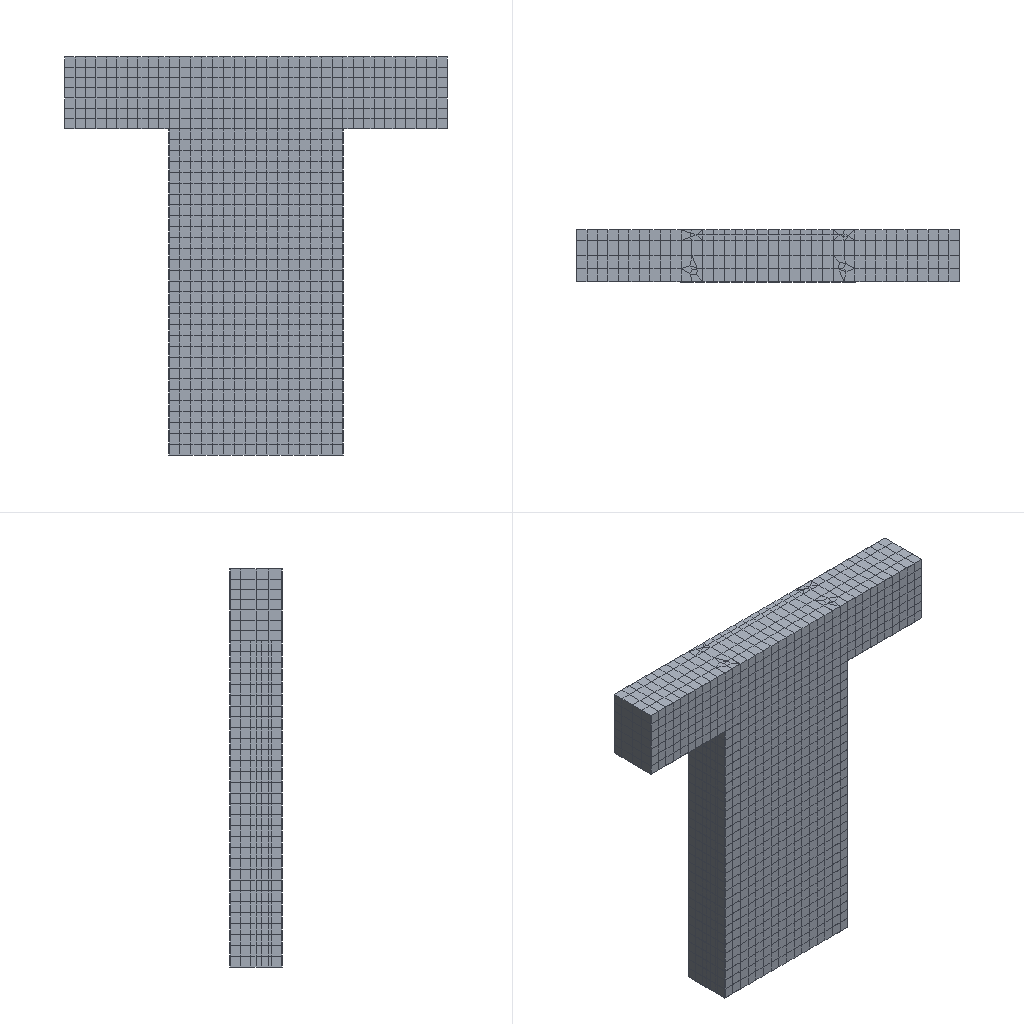Simulation study | abaqus
Set-up summary:
category,name,step,type,value,unit,region
solver,abaqus
solver,version,,,Abaqus/Standard 2020
units,not stated in the deck,,not stated
analysis,deck,,static,static
load_step,Step-1,Step-1,static
load_step,Step-2,Step-2,static
load_step,requested,,,2
mesh,nodes,,,11062
mesh,elements,,,8420
element_type,C3D6,,solid,444
element_type,R3D4,,rigid,1002
element_type,T3D2,,truss,2018
element_type,C3D8R,,solid,4956
load,load commands in deck,,count,2
bc,support commands in deck,,count,7
material,CON,,in results
material,Q235,,in results
check,setup vs results,,match,"per instance, exact: element labels, types and connectivity; labels of the nodes the elements use; coordinates of those nodes at SINGLE_PRECISION in 3 of 6 instance(s)"
Abaqus input file, long lists of numbers shortened:
*Heading
** Job name: Job-2 Model name: Model-1-Copy
** Generated by: Abaqus/CAE 2020
*Preprint, echo=NO, model=NO, history=NO, contact=NO
**
** PARTS
**
*Part, name=ban1
*Node
      1,         189.,         220.,           0.
      2,         189.,        -180.,           0.
** (494 more lines like these left out)
*Element, type=R3D4
1,  1, 13, 24,  4
2, 13, 14, 23, 24
** (499 more lines like these left out)
*Node
    497,         189.,          20.,          -5.
*Nset, nset=ban1-RefPt_, internal
497,
*Elset, elset=ban1, generate
   1,  501,    1
*End Part
**
*Part, name=ban2
*Node
      1,         189.,         220.,        1835.
      2,         189.,        -180.,        1835.
** (494 more lines like these left out)
*Element, type=R3D4
1,  1, 13, 24,  4
2, 13, 14, 23, 24
** (499 more lines like these left out)
*Node
    497,         189.,          20.,        1830.
*Nset, nset=ban2-RefPt_, internal
497,
*Elset, elset=ban2, generate
   1,  501,    1
*End Part
**
*Part, name=con
*Node
      1,         489.,          90.,        1500.
      2,        -111.,          90.,        1500.
** (5932 more lines like these left out)
*Element, type=C3D8R
  1,    5, 1585,  129,    1, 1654, 3925, 3903, 1653
  2, 1585, 1586,  130,  129, 3925, 3926, 3904, 3903
** (3814 more lines like these left out)
*Element, type=C3D6
1093,    5,   23,    1,  345,  546,  307
1094, 2438,   27,   28, 4466,  439,  547
** (442 more lines like these left out)
*Nset, nset=Set-12
    1,    2,    3,    4,    5,    6,    7,    8,    9,   10,   11,   12,   13,   14,   15,   16
   17,   18,   19,   20,   21,   22,   23,   24,   25,   26,   27,   28,   29,   30,   31,   32
** (360 more lines like these left out)
*Elset, elset=Set-12
    1,    2,    3,    4,    5,    6,    7,    8,    9,   10,   11,   12,   13,   14,   15,   16
   17,   18,   19,   20,   21,   22,   23,   24,   25,   26,   27,   28,   29,   30,   31,   32
** (249 more lines like these left out)
*Nset, nset=Set-14, generate
    1,  5934,     1
*Elset, elset=Set-14, generate
    1,  4260,     1
** Section: con
*Solid Section, elset=Set-14, material=con
,
*End Part
**
*Part, name=fiber
*Node
      1,         734.,          52.,        1525.
      2,         734.,         115.,        1525.
** (1652 more lines like these left out)
*Element, type=T3D2
1, 2, 1
2,   3, 873
** (2016 more lines like these left out)
*Nset, nset=Set-3, generate
    1,  1654,     1
*Elset, elset=Set-3, generate
    1,  2018,     1
*Nset, nset=nei
    1,    2,    3,    4,    5,    6,    7,    8,    9,   10,   11,   12,   13,   14,   15,   16
   17,   18,   19,   20,   21,   22,   23,   24,   25,   26,   27,   28,   29,   30,   31,   32
** (39 more lines like these left out)
*Elset, elset=nei
    1,    2,    3,    4,    5,    6,    7,    8,    9,   10,   11,   12,   13,   14,   15,   16
   17,   18,   19,   20,   21,   22,   23,   24,   25,   26,   27,   28,   29,   30,   31,   32
** (45 more lines like these left out)
** Section: fiber
*Solid Section, elset=Set-3, material=q235
12.56,
*End Part
**
*Part, name=liang1
*Node
      1,         588.,         140.,        1500.
      2,         588.,         140.,           0.
** (1238 more lines like these left out)
*Element, type=C3D8R
 1,   8, 145, 922, 176,   1,  57, 893, 116
 2, 145, 144, 923, 922,  57,  58, 894, 893
** (568 more lines like these left out)
*Nset, nset=Set-1, generate
    1,  1240,     1
*Elset, elset=Set-1, generate
   1,  570,    1
** Section: liang
*Solid Section, elset=Set-1, material=q235
,
*End Part
**
*Part, name=liang2
*Node
      1,        -112.,         -99.,           0.
      2,        -112.,         -99.,        1500.
** (1238 more lines like these left out)
*Element, type=C3D8R
 1, 174, 893, 922, 173,   1,  57, 114,   4
 2, 893, 894, 923, 922,  57,  58, 113, 114
** (568 more lines like these left out)
*Nset, nset=Set-1, generate
    1,  1240,     1
*Elset, elset=Set-1, generate
   1,  570,    1
** Section: liang
*Solid Section, elset=Set-1, material=q235
,
*End Part
**
**
** ASSEMBLY
**
*Assembly, name=Assembly
**
*Instance, name=ban1-1, part=ban1
*End Instance
**
*Instance, name=ban2-1, part=ban2
*End Instance
**
*Instance, name=con-1, part=con
*End Instance
**
*Instance, name=fiber-1, part=fiber
*End Instance
**
*Instance, name=liang1-1, part=liang1
*End Instance
**
*Instance, name=liang2-1, part=liang2
*End Instance
**
*Nset, nset=Set-4, instance=ban2-1
 497,
*Nset, nset=Set-5, instance=ban1-1
 497,
*Nset, nset=Set-6, instance=ban1-1
 497,
*Nset, nset=insert, instance=fiber-1
    1,    2,    3,    4,    5,    6,    7,    8,    9,   10,   11,   12,   13,   14,   15,   16
   17,   18,   19,   20,   21,   22,   23,   24,   25,   26,   27,   28,   29,   30,   31,   32
** (42 more lines like these left out)
*Nset, nset=m_Set-6, instance=fiber-1
    1,    2,    3,    4,    5,    6,    7,    8,    9,   10,   11,   12,   13,   14,   15,   16
   17,   18,   19,   20,   21,   22,   23,   24,   25,   26,   27,   28,   29,   30,   31,   32
** (40 more lines like these left out)
*Elset, elset=m_Set-6, instance=fiber-1
    1,    2,    3,    4,    5,    6,    7,    8,    9,   10,   11,   12,   13,   14,   15,   16
   17,   18,   19,   20,   21,   22,   23,   24,   25,   26,   27,   28,   29,   30,   31,   32
** (48 more lines like these left out)
*Nset, nset=m_Set-8, instance=fiber-1
    1,    2,    3,    4,    5,    6,    7,    8,    9,   10,   11,   12,   13,   14,   15,   16
   17,   18,   19,   20,   21,   22,   23,   24,   25,   26,   27,   28,   29,   30,   31,   32
** (38 more lines like these left out)
*Elset, elset=m_Set-8, instance=fiber-1
    1,    2,    3,    4,    5,    6,    7,    8,    9,   10,   11,   12,   13,   14,   15,   16
   17,   18,   19,   20,   21,   22,   23,   24,   25,   26,   27,   28,   29,   30,   31,   32
** (45 more lines like these left out)
*Nset, nset=m_Set-10, instance=fiber-1
    1,    2,    3,    4,    5,    6,    7,    8,    9,   10,   11,   12,   13,   14,   15,   16
   17,   18,   19,   20,   21,   22,   23,   24,   25,   26,   27,   28,   29,   30,   31,   32
** (38 more lines like these left out)
*Elset, elset=m_Set-10, instance=fiber-1
    1,    2,    3,    4,    5,    6,    7,    8,    9,   10,   11,   12,   13,   14,   15,   16
   17,   18,   19,   20,   21,   22,   23,   24,   25,   26,   27,   28,   29,   30,   31,   32
** (45 more lines like these left out)
*Nset, nset=m_Set-12, instance=fiber-1
    1,    2,    3,    4,    5,    6,    7,    8,    9,   10,   11,   12,   13,   14,   15,   16
   17,   18,   19,   20,   21,   22,   23,   24,   25,   26,   27,   28,   29,   30,   31,   32
** (91 more lines like these left out)
*Elset, elset=m_Set-12, instance=fiber-1
    1,    2,    3,    4,    5,    6,    7,    8,    9,   10,   11,   12,   13,   14,   15,   16
   17,   18,   19,   20,   21,   22,   23,   24,   25,   26,   27,   28,   29,   30,   31,   32
** (110 more lines like these left out)
*Nset, nset=s_Set-6, instance=con-1
    1,    2,    3,    4,    5,    6,    7,    8,    9,   10,   11,   12,   13,   14,   15,   16
   17,   18,   19,   20,   21,   22,   23,   24,   25,   26,   27,   28,   29,   30,   31,   32
** (360 more lines like these left out)
*Elset, elset=s_Set-6, instance=con-1
    1,    2,    3,    4,    5,    6,    7,    8,    9,   10,   11,   12,   13,   14,   15,   16
   17,   18,   19,   20,   21,   22,   23,   24,   25,   26,   27,   28,   29,   30,   31,   32
** (249 more lines like these left out)
*Nset, nset=s_Set-10, instance=con-1, generate
    1,  5934,     1
*Elset, elset=s_Set-10, instance=con-1, generate
    1,  4260,     1
*Nset, nset=s_Set-12, instance=con-1, generate
    1,  5934,     1
*Elset, elset=s_Set-12, instance=con-1, generate
    1,  4260,     1
*Elset, elset=_m_Surf-1_SPOS, internal, instance=ban1-1
   8,   9,  10,  11,  12,  13,  14,  15,  16,  17,  18,  19,  20,  21,  22,  23
  24,  25,  26,  27,  28,  29,  30,  31,  32,  33,  34,  35,  36,  37,  38,  39
** (12 more lines like these left out)
*Surface, type=ELEMENT, name=m_Surf-1
_m_Surf-1_SPOS, SPOS
*Elset, elset=_m_Surf-3_SPOS, internal, instance=ban2-1
 128, 129, 130, 131, 132, 133, 134, 135, 136, 137, 138, 139, 140, 141, 142, 143
 144, 145, 146, 147, 148, 149, 150, 151, 152, 153, 154, 155, 156, 157, 158, 159
** (12 more lines like these left out)
*Surface, type=ELEMENT, name=m_Surf-3
_m_Surf-3_SPOS, SPOS
*Elset, elset=_m_Surf-5_S1, internal, instance=con-1, generate
 3670,  3673,     1
*Elset, elset=_m_Surf-5_S5, internal, instance=con-1
  444,  468,  492,  516,  540,  564,  588,  612,  636,  660,  684,  708,  732,  756,  780,  804
  828,  852,  876,  900,  924,  948,  972,  996, 1020, 1044, 1068, 1092, 2104, 2164, 2200, 2208
** (4 more lines like these left out)
*Elset, elset=_m_Surf-5_S4, internal, instance=con-1
 2193, 2198, 2201, 2206, 2209, 2214, 2217, 2222, 2225, 2230, 2233, 2238, 2241, 2246, 2249, 2254
 2257, 2262, 2265, 2270, 2273, 2278, 2281, 2286, 2289, 2294, 2297, 2302, 2305, 2310, 2313, 2318
** (10 more lines like these left out)
*Elset, elset=_m_Surf-5_S3, internal, instance=con-1
 2197, 2205, 2213, 2221, 2229, 2237, 2245, 2253, 2261, 2269, 2277, 2285, 2293, 2301, 2309, 2317
 2325, 2333, 2341, 2349, 2357, 2365, 2373, 2381, 2389, 2397, 2405, 2413, 2418, 2422, 2426, 2430
** (2 more lines like these left out)
*Elset, elset=_m_Surf-5_S6, internal, instance=con-1
 1396, 1420, 1444, 1468, 1492, 1516, 1540, 1564, 1588, 1612, 1636, 1660, 1684, 1708, 1732, 1756
 1780, 1804, 1828, 1852, 1876, 1900, 1924, 1948, 1972, 1996, 2020, 2044, 2068, 2128, 2197, 2199
** (4 more lines like these left out)
*Surface, type=ELEMENT, name=m_Surf-5
_m_Surf-5_S1, S1
_m_Surf-5_S5, S5
_m_Surf-5_S4, S4
_m_Surf-5_S6, S6
_m_Surf-5_S3, S3
*Elset, elset=_m_Surf-7_S2, internal, instance=liang1-1
   1,   2,   3,   4,   5,   6,   7,   8,   9,  10,  11,  12,  13,  14,  15,  16
  17,  18,  19,  20,  21,  22,  23,  24,  25,  26,  27,  28,  29,  30,  31,  32
** (6 more lines like these left out)
*Elset, elset=_m_Surf-7_S5, internal, instance=liang1-1
 151, 152, 153, 154, 155, 156, 157, 158, 159, 160, 161, 162, 163, 164, 165, 166
 167, 168, 169, 170, 171, 172, 173, 174, 175, 176, 177, 178, 179, 180, 181, 182
** (6 more lines like these left out)
*Elset, elset=_m_Surf-7_S4, internal, instance=liang1-1
  61,  62,  63,  64,  65,  66,  67,  68,  69,  70,  71,  72,  73,  74,  75,  76
  77,  78,  79,  80,  81,  82,  83,  84,  85,  86,  87,  88,  89,  90, 270, 390
*Elset, elset=_m_Surf-7_S6, internal, instance=liang1-1
 241, 361
*Elset, elset=_m_Surf-7_S1, internal, instance=liang1-1
 241, 242, 243, 244, 245, 246, 247, 248, 249, 250, 251, 252, 253, 254, 255, 256
 257, 258, 259, 260, 261, 262, 263, 264, 265, 266, 267, 268, 269, 270, 541, 542
** (2 more lines like these left out)
*Elset, elset=_m_Surf-7_S3, internal, instance=liang1-1, generate
 361,  540,    1
*Surface, type=ELEMENT, name=m_Surf-7
_m_Surf-7_S2, S2
_m_Surf-7_S5, S5
_m_Surf-7_S4, S4
_m_Surf-7_S6, S6
_m_Surf-7_S1, S1
_m_Surf-7_S3, S3
*Elset, elset=_m_Surf-9_S6, internal, instance=con-1
 2194, 2202, 2210, 2218, 2226, 2234, 2242, 2250, 2258, 2266, 2274, 2282, 2290, 2298, 2306, 2314
 2322, 2330, 2338, 2346, 2354, 2362, 2370, 2378, 2386, 2394, 2402, 2410, 2531, 2535, 2539, 2543
** (4 more lines like these left out)
*Elset, elset=_m_Surf-9_S3, internal, instance=con-1
 2199, 2207, 2215, 2223, 2231, 2239, 2247, 2255, 2263, 2271, 2279, 2287, 2295, 2303, 2311, 2319
 2327, 2335, 2343, 2351, 2359, 2367, 2375, 2383, 2391, 2399, 2407, 2415, 2646, 2653, 2660, 2667
*Surface, type=ELEMENT, name=m_Surf-9
_m_Surf-9_S6, S6
_m_Surf-9_S3, S3
*Elset, elset=_m_Surf-11_S6, internal, instance=con-1
 2711, 2719, 2727, 2735, 2743, 2751, 2759, 2767, 2775, 2783, 2791, 2799, 2807, 2815, 2823, 2831
 2839, 2847, 2855, 2863, 2871, 2879, 2887, 2895, 2903, 2911, 2919, 2927, 2935, 2949, 2973, 2974
** (2 more lines like these left out)
*Elset, elset=_m_Surf-11_S3, internal, instance=con-1
 2709, 2717, 2725, 2733, 2741, 2749, 2757, 2765, 2773, 2781, 2789, 2797, 2805, 2813, 2821, 2829
 2837, 2845, 2853, 2861, 2869, 2877, 2885, 2893, 2901, 2909, 2917, 2925, 2933, 2940, 2947, 2954
*Elset, elset=_m_Surf-11_S4, internal, instance=con-1
 1094, 1100, 1106, 1112, 1118, 1124, 1130, 1136, 1142, 1148, 1154, 1160, 1166, 1172, 1178, 1184
 1190, 1196, 1202, 1208, 1214, 1220, 1226, 1232, 1238, 1244, 1250, 1256, 2961, 2968
*Surface, type=ELEMENT, name=m_Surf-11
_m_Surf-11_S6, S6
_m_Surf-11_S3, S3
_m_Surf-11_S4, S4
*Elset, elset=_m_Surf-14_S1, internal, instance=con-1
 3653, 3654, 3655, 3656, 3670, 3671, 3672, 3673
*Elset, elset=_m_Surf-14_S5, internal, instance=con-1
  444,  468,  492,  516,  540,  564,  588,  612,  636,  660,  684,  708,  732,  756,  780,  804
  828,  852,  876,  900,  924,  948,  972,  996, 1020, 1044, 1068, 1092, 2104, 2164, 2200, 2208
** (4 more lines like these left out)
*Elset, elset=_m_Surf-14_S4, internal, instance=con-1
 2193, 2198, 2201, 2206, 2209, 2214, 2217, 2222, 2225, 2230, 2233, 2238, 2241, 2246, 2249, 2254
 2257, 2262, 2265, 2270, 2273, 2278, 2281, 2286, 2289, 2294, 2297, 2302, 2305, 2310, 2313, 2318
** (10 more lines like these left out)
*Elset, elset=_m_Surf-14_S3, internal, instance=con-1
 2197, 2205, 2213, 2221, 2229, 2237, 2245, 2253, 2261, 2269, 2277, 2285, 2293, 2301, 2309, 2317
 2325, 2333, 2341, 2349, 2357, 2365, 2373, 2381, 2389, 2397, 2405, 2413, 2418, 2422, 2426, 2430
** (2 more lines like these left out)
*Elset, elset=_m_Surf-14_S6, internal, instance=con-1
 1396, 1420, 1444, 1468, 1492, 1516, 1540, 1564, 1588, 1612, 1636, 1660, 1684, 1708, 1732, 1756
 1780, 1804, 1828, 1852, 1876, 1900, 1924, 1948, 1972, 1996, 2020, 2044, 2068, 2128, 2197, 2199
** (4 more lines like these left out)
*Surface, type=ELEMENT, name=m_Surf-14
_m_Surf-14_S1, S1
_m_Surf-14_S5, S5
_m_Surf-14_S4, S4
_m_Surf-14_S6, S6
_m_Surf-14_S3, S3
*Elset, elset=_s_Surf-1_S2, internal, instance=con-1, generate
 361,  420,    1
*Surface, type=ELEMENT, name=s_Surf-1
_s_Surf-1_S2, S2
*Elset, elset=_s_Surf-3_S5, internal, instance=con-1
 3001, 3023, 3045, 3067, 3089, 3111, 3133, 3241, 3244, 3283, 3286, 3325, 3328, 3367, 3370, 3409
 3412, 3451, 3454, 3493, 3496, 3535, 3538, 3577, 3580, 3619, 3622, 3878, 3880, 3920, 3922, 3962
** (1 more lines like these left out)
*Elset, elset=_s_Surf-3_S3, internal, instance=con-1
 3002, 3024, 3046, 3068, 3090, 3112, 3134, 3242, 3243, 3245, 3284, 3285, 3287, 3326, 3327, 3329
 3368, 3369, 3371, 3410, 3411, 3413, 3452, 3453, 3455, 3494, 3495, 3497, 3536, 3537, 3539, 3578
** (3 more lines like these left out)
*Elset, elset=_s_Surf-3_S2, internal, instance=con-1, generate
 2105,  2164,     1
*Elset, elset=_s_Surf-3_S4, internal, instance=con-1
 3240, 3282, 3324, 3366, 3408, 3450, 3492, 3534, 3576, 3618, 3882, 3924, 3966, 4008, 4050, 4092
 4134, 4176, 4218, 4260
*Surface, type=ELEMENT, name=s_Surf-3
_s_Surf-3_S5, S5
_s_Surf-3_S3, S3
_s_Surf-3_S2, S2
_s_Surf-3_S4, S4
*Elset, elset=_s_Surf-5_S4, internal, instance=liang2-1
  30,  60,  90, 120, 181, 182, 183, 184, 185, 186, 187, 188, 189, 190, 191, 192
 193, 194, 195, 196, 197, 198, 199, 200, 201, 202, 203, 204, 205, 206, 207, 208
** (1 more lines like these left out)
*Elset, elset=_s_Surf-5_S6, internal, instance=liang2-1
  91, 151, 152, 153, 154, 155, 156, 157, 158, 159, 160, 161, 162, 163, 164, 165
 166, 167, 168, 169, 170, 171, 172, 173, 174, 175, 176, 177, 178, 179, 180, 181
** (3 more lines like these left out)
*Elset, elset=_s_Surf-5_S2, internal, instance=liang2-1
  91,  92,  93,  94,  95,  96,  97,  98,  99, 100, 101, 102, 103, 104, 105, 106
 107, 108, 109, 110, 111, 112, 113, 114, 115, 116, 117, 118, 119, 120, 151, 271
** (8 more lines like these left out)
*Elset, elset=_s_Surf-5_S3, internal, instance=liang2-1
   1,   2,   3,   4,   5,   6,   7,   8,   9,  10,  11,  12,  13,  14,  15,  16
  17,  18,  19,  20,  21,  22,  23,  24,  25,  26,  27,  28,  29,  30,  31,  32
** (4 more lines like these left out)
*Elset, elset=_s_Surf-5_S5, internal, instance=liang2-1
  91,  92,  93,  94,  95,  96,  97,  98,  99, 100, 101, 102, 103, 104, 105, 106
 107, 108, 109, 110, 111, 112, 113, 114, 115, 116, 117, 118, 119, 120, 151, 152
** (8 more lines like these left out)
*Elset, elset=_s_Surf-5_S1, internal, instance=liang2-1
  91,  92,  93,  94,  95,  96,  97,  98,  99, 100, 101, 102, 103, 104, 105, 106
 107, 108, 109, 110, 111, 112, 113, 114, 115, 116, 117, 118, 119, 120, 180, 211
** (6 more lines like these left out)
*Surface, type=ELEMENT, name=s_Surf-5
_s_Surf-5_S4, S4
_s_Surf-5_S6, S6
_s_Surf-5_S2, S2
_s_Surf-5_S3, S3
_s_Surf-5_S5, S5
_s_Surf-5_S1, S1
*Elset, elset=_s_Surf-7_S1, internal, instance=con-1, generate
 3001,  3008,     1
*Elset, elset=_s_Surf-7_S3, internal, instance=con-1
  433,  457,  481,  505,  529,  553,  577,  601,  625,  649,  673,  697,  721,  745,  769,  793
  817,  841,  865,  889,  913,  937,  961,  985, 1009, 1033, 1057, 1081, 1093, 1099, 1105, 1111
** (4 more lines like these left out)
*Elset, elset=_s_Surf-7_S4, internal, instance=con-1
 1095, 1101, 1107, 1113, 1119, 1125, 1131, 1137, 1143, 1149, 1155, 1161, 1167, 1173, 1179, 1185
 1191, 1197, 1203, 1209, 1215, 1221, 1227, 1233, 1239, 1245, 1251, 1257, 1262, 1266, 1270, 1274
** (6 more lines like these left out)
*Elset, elset=_s_Surf-7_S5, internal, instance=con-1
 1095, 1101, 1107, 1113, 1119, 1125, 1131, 1137, 1143, 1149, 1155, 1161, 1167, 1173, 1179, 1185
 1191, 1197, 1203, 1209, 1215, 1221, 1227, 1233, 1239, 1245, 1251, 1257, 1263, 1264, 1267, 1268
** (8 more lines like these left out)
*Elset, elset=_s_Surf-7_S6, internal, instance=con-1
 2707, 2713, 2715, 2721, 2723, 2729, 2731, 2737, 2739, 2745, 2747, 2753, 2755, 2761, 2763, 2769
 2771, 2777, 2779, 2785, 2787, 2793, 2795, 2801, 2803, 2809, 2811, 2817, 2819, 2825, 2827, 2833
** (2 more lines like these left out)
*Surface, type=ELEMENT, name=s_Surf-7
_s_Surf-7_S1, S1
_s_Surf-7_S3, S3
_s_Surf-7_S4, S4
_s_Surf-7_S6, S6
_s_Surf-7_S5, S5
*Elset, elset=_s_Surf-9_S3, internal, instance=liang2-1, generate
 391,  540,    1
*Surface, type=ELEMENT, name=s_Surf-9
_s_Surf-9_S3, S3
*Elset, elset=_s_Surf-11_S3, internal, instance=liang1-1, generate
 391,  540,    1
*Surface, type=ELEMENT, name=s_Surf-11
_s_Surf-11_S3, S3
*Elset, elset=_s_Surf-13_S2, internal, instance=con-1, generate
 361,  420,    1
*Elset, elset=_s_Surf-13_S2, internal, instance=liang1-1
 61,
*Elset, elset=_s_Surf-13_S4, internal, instance=liang1-1
  30,  60, 360, 420, 450, 480, 510, 540
*Elset, elset=_s_Surf-13_S4, internal, instance=liang2-1
 120, 300, 330, 390
*Elset, elset=_s_Surf-13_S1, internal, instance=liang1-1
 120, 150
*Elset, elset=_s_Surf-13_S1, internal, instance=liang2-1
 150, 180
*Elset, elset=_s_Surf-13_S6, internal, instance=liang1-1
 151, 181, 211, 241, 271, 301, 361
*Elset, elset=_s_Surf-13_S6, internal, instance=liang2-1
   1,  31,  61, 211, 241, 331, 391, 421, 451, 481, 511
*Elset, elset=_s_Surf-13_S5, internal, instance=liang1-1
 570,
*Elset, elset=_s_Surf-13_S3, internal, instance=liang2-1
 181, 541
*Surface, type=ELEMENT, name=s_Surf-13
_s_Surf-13_S2, S2
_s_Surf-13_S4, S4
_s_Surf-13_S6, S6
_s_Surf-13_S1, S1
_s_Surf-13_S5, S5
_s_Surf-13_S3, S3
*Elset, elset=_s_Surf-15_S2, internal, instance=con-1
  361,  362,  363,  364,  365,  366,  367,  368,  369,  370,  371,  372,  373,  374,  375,  376
  377,  378,  379,  380,  381,  382,  383,  384,  385,  386,  387,  388,  389,  390,  391,  392
** (6 more lines like these left out)
*Elset, elset=_s_Surf-15_S4, internal, instance=con-1
 3240, 3282, 3324, 3366, 3408, 3450, 3492, 3534, 3576, 3618, 3882, 3924, 3966, 4008, 4050, 4092
 4134, 4176, 4218, 4260
*Elset, elset=_s_Surf-15_S5, internal, instance=con-1
 3241, 3244, 3283, 3286, 3325, 3328, 3367, 3370, 3409, 3412, 3451, 3454, 3493, 3496, 3535, 3538
 3577, 3580, 3619, 3622, 3878, 3880, 3920, 3922, 3962, 3964, 4004, 4006, 4046, 4048, 4088, 4090
** (1 more lines like these left out)
*Elset, elset=_s_Surf-15_S3, internal, instance=con-1
 3242, 3243, 3245, 3284, 3285, 3287, 3326, 3327, 3329, 3368, 3369, 3371, 3410, 3411, 3413, 3452
 3453, 3455, 3494, 3495, 3497, 3536, 3537, 3539, 3578, 3579, 3581, 3620, 3621, 3623, 3877, 3879
** (2 more lines like these left out)
*Surface, type=ELEMENT, name=s_Surf-15
_s_Surf-15_S2, S2
_s_Surf-15_S4, S4
_s_Surf-15_S5, S5
_s_Surf-15_S3, S3
*Elset, elset=_s_Surf-16_S2, internal, instance=con-1
 2105, 2106, 2107, 2108, 2109, 2110, 2111, 2112, 2113, 2114, 2115, 2116, 2117, 2118, 2119, 2120
 2121, 2122, 2123, 2124, 2125, 2126, 2127, 2128, 2129, 2130, 2131, 2132, 2133, 2134, 2135, 2136
** (5 more lines like these left out)
*Elset, elset=_s_Surf-16_S2, internal, instance=liang1-1
 61,
*Elset, elset=_s_Surf-16_S4, internal, instance=liang1-1
  30,  60, 360, 420, 450, 480, 510, 540
*Elset, elset=_s_Surf-16_S4, internal, instance=liang2-1
 120, 300, 330, 390
*Elset, elset=_s_Surf-16_S1, internal, instance=liang1-1
 120, 150
*Elset, elset=_s_Surf-16_S1, internal, instance=liang2-1
 150, 180
*Elset, elset=_s_Surf-16_S6, internal, instance=liang1-1
 151, 181, 211, 241, 271, 301, 361
*Elset, elset=_s_Surf-16_S6, internal, instance=liang2-1
   1,  31,  61, 211, 241, 331, 391, 421, 451, 481, 511
*Elset, elset=_s_Surf-16_S5, internal, instance=liang1-1
 570,
*Elset, elset=_s_Surf-16_S3, internal, instance=liang2-1
 181, 541
*Surface, type=ELEMENT, name=s_Surf-16
_s_Surf-16_S2, S2
_s_Surf-16_S4, S4
_s_Surf-16_S6, S6
_s_Surf-16_S1, S1
_s_Surf-16_S5, S5
_s_Surf-16_S3, S3
*Elset, elset=_s_Surf-17_S3, internal, instance=liang2-1, generate
 391,  540,    1
*Surface, type=ELEMENT, name=s_Surf-17
_s_Surf-17_S3, S3
*Elset, elset=_s_Surf-18_S2, internal, instance=con-1
 2105, 2106, 2107, 2108, 2109, 2110, 2111, 2112, 2113, 2114, 2115, 2116, 2117, 2118, 2119, 2120
 2121, 2122, 2123, 2124, 2125, 2126, 2127, 2128, 2129, 2130, 2131, 2132, 2133, 2134, 2135, 2136
** (5 more lines like these left out)
*Elset, elset=_s_Surf-18_S2, internal, instance=liang1-1
 61,
*Elset, elset=_s_Surf-18_S4, internal, instance=liang1-1
  30,  60, 360, 420, 450, 480, 510, 540
*Elset, elset=_s_Surf-18_S4, internal, instance=liang2-1
 120, 300, 330, 390
*Elset, elset=_s_Surf-18_S1, internal, instance=liang1-1
 120, 150
*Elset, elset=_s_Surf-18_S1, internal, instance=liang2-1
 150, 180
*Elset, elset=_s_Surf-18_S6, internal, instance=liang1-1
 151, 181, 211, 241, 271, 301, 361
*Elset, elset=_s_Surf-18_S6, internal, instance=liang2-1
   1,  31,  61, 211, 241, 331, 391, 421, 451, 481, 511
*Elset, elset=_s_Surf-18_S5, internal, instance=liang1-1
 570,
*Elset, elset=_s_Surf-18_S3, internal, instance=liang2-1
 181, 541
*Surface, type=ELEMENT, name=s_Surf-18
_s_Surf-18_S2, S2
_s_Surf-18_S4, S4
_s_Surf-18_S6, S6
_s_Surf-18_S1, S1
_s_Surf-18_S5, S5
_s_Surf-18_S3, S3
*Elset, elset=_s_Surf-19_S2, internal, instance=con-1
  361,  362,  363,  364,  365,  366,  367,  368,  369,  370,  371,  372,  373,  374,  375,  376
  377,  378,  379,  380,  381,  382,  383,  384,  385,  386,  387,  388,  389,  390,  391,  392
** (6 more lines like these left out)
*Elset, elset=_s_Surf-19_S4, internal, instance=con-1
 3240, 3282, 3324, 3366, 3408, 3450, 3492, 3534, 3576, 3618, 3882, 3924, 3966, 4008, 4050, 4092
 4134, 4176, 4218, 4260
*Elset, elset=_s_Surf-19_S5, internal, instance=con-1
 3241, 3244, 3283, 3286, 3325, 3328, 3367, 3370, 3409, 3412, 3451, 3454, 3493, 3496, 3535, 3538
 3577, 3580, 3619, 3622, 3878, 3880, 3920, 3922, 3962, 3964, 4004, 4006, 4046, 4048, 4088, 4090
** (1 more lines like these left out)
*Elset, elset=_s_Surf-19_S3, internal, instance=con-1
 3242, 3243, 3245, 3284, 3285, 3287, 3326, 3327, 3329, 3368, 3369, 3371, 3410, 3411, 3413, 3452
 3453, 3455, 3494, 3495, 3497, 3536, 3537, 3539, 3578, 3579, 3581, 3620, 3621, 3623, 3877, 3879
** (2 more lines like these left out)
*Surface, type=ELEMENT, name=s_Surf-19
_s_Surf-19_S2, S2
_s_Surf-19_S4, S4
_s_Surf-19_S5, S5
_s_Surf-19_S3, S3
*Rigid Body, ref node=ban1-1.ban1-RefPt_, elset=ban1-1.ban1
*Rigid Body, ref node=ban2-1.ban2-RefPt_, elset=ban2-1.ban2
** Constraint: Constraint-4
*Tie, name=Constraint-4, adjust=yes
s_Surf-11, m_Surf-11
** Constraint: Constraint-ban1
*Tie, name=Constraint-ban1, adjust=yes
s_Surf-18, m_Surf-1
** Constraint: Constraint-ban2
*Tie, name=Constraint-ban2, adjust=yes
s_Surf-19, m_Surf-3
** Constraint: Constraint-liang
*Tie, name=Constraint-liang, adjust=yes
m_Surf-9, s_Surf-17
** Constraint: Constraint-nei
*Embedded Element, host elset=s_Set-12
m_Set-12
*End Assembly
*Amplitude, name=Amp-1
             0.,              0.,              1.,              1.
*Amplitude, name=Amp-load
             0.,              0.,             0.5,             0.1,              1.,            -0.1,             1.5,              0.
             2.,             0.4,             2.5,            -0.4,              3.,              0.,             3.5,             0.6
             4.,            -0.6,             4.5,              0.,              5.,             0.9,             5.5,            -0.9
             6.,              0.,             6.5,              1.,              7.,             -1.,             7.5,              0.
             8.,             1.3,             8.5,            -1.3,              9.,              0.,             9.5,             1.6
            10.,            -1.6,            10.5,              0.,             11.,             1.9,            11.5,            -1.9
            12.,              0.,            12.5,             2.4,             13.,            -2.4,            13.5,              0.
            14.,             2.8,            14.5,            -2.8,             15.,              0.,            15.5,             3.2
            16.,            -3.2,            16.5,              0.,             17.,             3.6,            17.5,            -3.6
            18.,              0.,            18.5,              4.,             19.,             -4.,            19.5,              0.
            20.,             4.4,            20.5,            -4.4,             21.,              0.,            21.5,             4.8
            22.,            -4.8,            22.5,              0.,             23.,             5.2,            23.5,            -5.2
            24.,              0.,            24.5,             5.6,             25.,            -5.6,            25.5,              0.
            26.,              6.,            26.5,             -6.,             27.,              0.,            27.5,             6.5
            28.,            -6.5,            28.5,              0.,             29.,              7.,            29.5,             -7.
            30.,              0.,            30.5,             7.5,             31.,            -7.5,            31.5,              0.
            32.,              8.,            32.5,             -8.,             33.,              0.,            33.5,             8.5
            34.,            -8.5,            34.5,              0.,             35.,              9.,            35.5,             -9.
            36.,              0.,            36.5,             9.6,             37.,            -9.6,            37.5,              0.
            38.,            10.2,            38.5,           -10.2,             39.,              0.,            39.5,            10.8
            40.,           -10.8,            40.5,              0.,             41.,            11.4,            41.5,           -11.4
            42.,              0.,            42.5,             12.,             43.,            -12.,            43.5,              0.
            44.,            12.7,            44.5,           -12.7,             45.,              0.,            45.5,            13.4
            46.,           -13.4,            46.5,              0.,             47.,            14.1,            47.5,           -14.1
            48.,              0.,            48.5,            14.9,             49.,           -14.9,            49.5,              0.
            50.,            15.7,            50.5,           -15.7,             51.,              0.,            51.5,            16.5
            52.,           -16.5,            52.5,              0.
**
** MATERIALS
**
*Material, name=con
*Elastic
2260., 0.2
*Concrete Damaged Plasticity
45.,     0.1,    1.16,  0.6667, 0.00075
*Concrete Compression Hardening
  2.669,         0.
  3.127, 0.001499
  3.503, 0.001799
 3.659, 0.001949
  3.795, 0.002099
 3.909, 0.002249
  4.003, 0.002399
 4.076,  0.002549
  4.128, 0.002699
 4.16, 0.002849
    4.17, 0.002999
  4.087,  0.003299
  4.003, 0.003599
  3.92, 0.003899
  3.836, 0.004199
   3.753, 0.004499
  3.67, 0.004799
*Concrete Tension Stiffening
   0.1984,         0.
   0.2325, 0.0015
   0.2604, 0.0018
 0.272, 0.00195
   0.2821, 0.0021
 0.2906, 0.00225
   0.2976, 0.0024
 0.303, 0.00255
   0.3069, 0.0027
 0.3092, 0.00285
     0.31, 0.003
   0.3038, 0.0033
   0.2976, 0.0036
   0.2914, 0.0039
   0.2852, 0.0042
    0.279, 0.0045
   0.2728, 0.0048
*Concrete Compression Damage
        0.,         0.
 0.0395, 0.001499
 0.07207, 0.001799
 0.08879, 0.001949
   0.1058, 0.002099
  0.1232, 0.002249
    0.1409, 0.002399
  0.159,  0.002549
  0.1775, 0.002699
  0.1964, 0.002849
  0.2158, 0.002999
  0.2598,  0.003299
  0.2985, 0.003599
  0.3331, 0.003899
  0.3643, 0.004199
  0.3925, 0.004499
  0.4184, 0.004799
*Concrete Tension Damage
       0.,         0.
 0.7381, 0.0015
 0.747, 0.0018
 0.7516, 0.00195
 0.7562, 0.0021
 0.7609, 0.00225
 0.7658, 0.0024
 0.7707, 0.00255
 0.7757, 0.0027
 0.7809, 0.00285
 0.7862, 0.003
 0.7982, 0.0033
 0.8087, 0.0036
 0.8182, 0.0039
 0.8267, 0.0042
 0.8344, 0.0045
  0.8414, 0.0048
*Material, name=q235
*Elastic
124500., 0.25
*Plastic
 50.,      0.
 80.,  0.0001
100.,  0.0005
180.,   0.001
250.,  0.0016
 80.,  0.0024
 40.,  0.0028
 10., 0.00323
**
** INTERACTION PROPERTIES
**
*Surface Interaction, name=IntProp-1
1.,
*Friction, slip tolerance=0.005
 0.2,
*Surface Behavior, pressure-overclosure=HARD
**
** INTERACTIONS
**
** Interaction: Int-1
*Contact Pair, interaction=IntProp-1, type=SURFACE TO SURFACE, adjust=1.
s_Surf-5, m_Surf-14
** Interaction: Int-2
*Contact Pair, interaction=IntProp-1, type=SURFACE TO SURFACE, adjust=1.
m_Surf-7, s_Surf-7
** ----------------------------------------------------------------
**
** STEP: Step-1
**
*Step, name=Step-1, nlgeom=NO, inc=1000
*Static
0.01, 1., 1e-05, 1.
**
** BOUNDARY CONDITIONS
**
** Name: [REDACTED] : Symmetric / antisymmetric / fully fixed
*Boundary
Set-4, ENCASTRE
**
** LOADS
**
** Name: Load   Type: Concentrated force
*Cload, amplitude=Amp-1
Set-5, 3, 259200.
**
** OUTPUT REQUESTS
**
*Restart, write, frequency=0
**
** FIELD OUTPUT: F-Output-1
**
*Output, field, variable=PRESELECT
*Output, history, frequency=0
*End Step
** ----------------------------------------------------------------
**
** STEP: Step-2
**
*Step, name=Step-2, nlgeom=NO, inc=5000
*Static
0.1, 54.5, 0.0001, 54.5
**
** BOUNDARY CONDITIONS
**
** Name: [REDACTED] : Displacement/rotation angle
*Boundary, amplitude=Amp-load
Set-6, 1, 1, 1.
Set-6, 2, 2
Set-6, 3, 3
Set-6, 4, 4
Set-6, 5, 5
Set-6, 6, 6
**
** OUTPUT REQUESTS
**
*Restart, write, frequency=0
**
** FIELD OUTPUT: F-Output-1
**
*Output, field
*Node Output
CF, RF, RM, RT, U, V
*Element Output, directions=YES
DAMAGEC, DAMAGET, E, LE, MISES, MISESMAX, MISESONLY, P, PE, PEEQ, PEEQMAX, PEEQT, PEMAG, S, SDEG, SF
SSAVG
*Contact Output
CDISP, CSTRESS
**
** HISTORY OUTPUT: H-Output-1
**
*Output, history
*Node Output, nset=Set-6
RF1, U1
*End Step
Results summary:
result,step,,completed,increments=11 time=1.0/1.0
result,step,,partial,increments=274 time=25.815/54.5
result,analysis,,,static
result,last_loadstep,,,2
result,primary field,,,U
result,reaction total,,FX,0.0,model units
result,reaction total,,FY,-3.1e-05,model units
result,reaction total,,FZ,-259200.0,model units